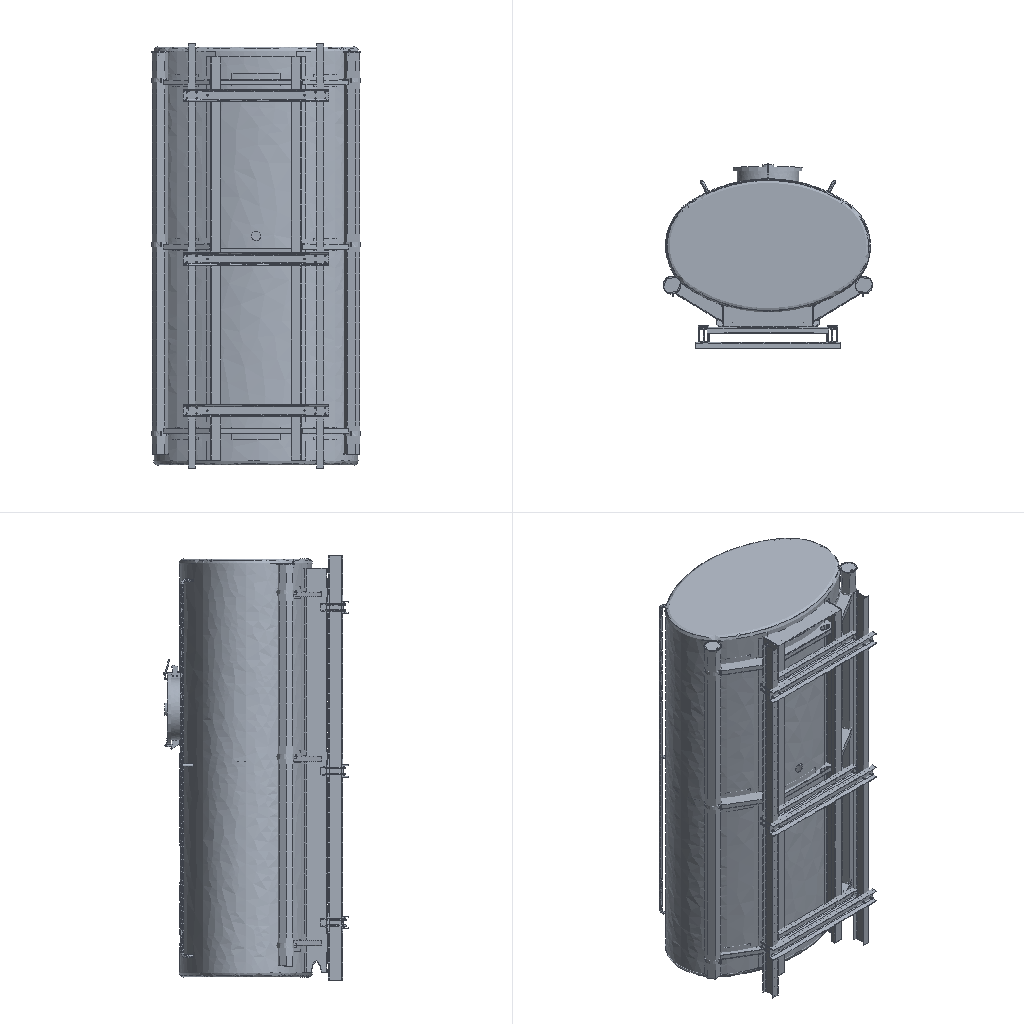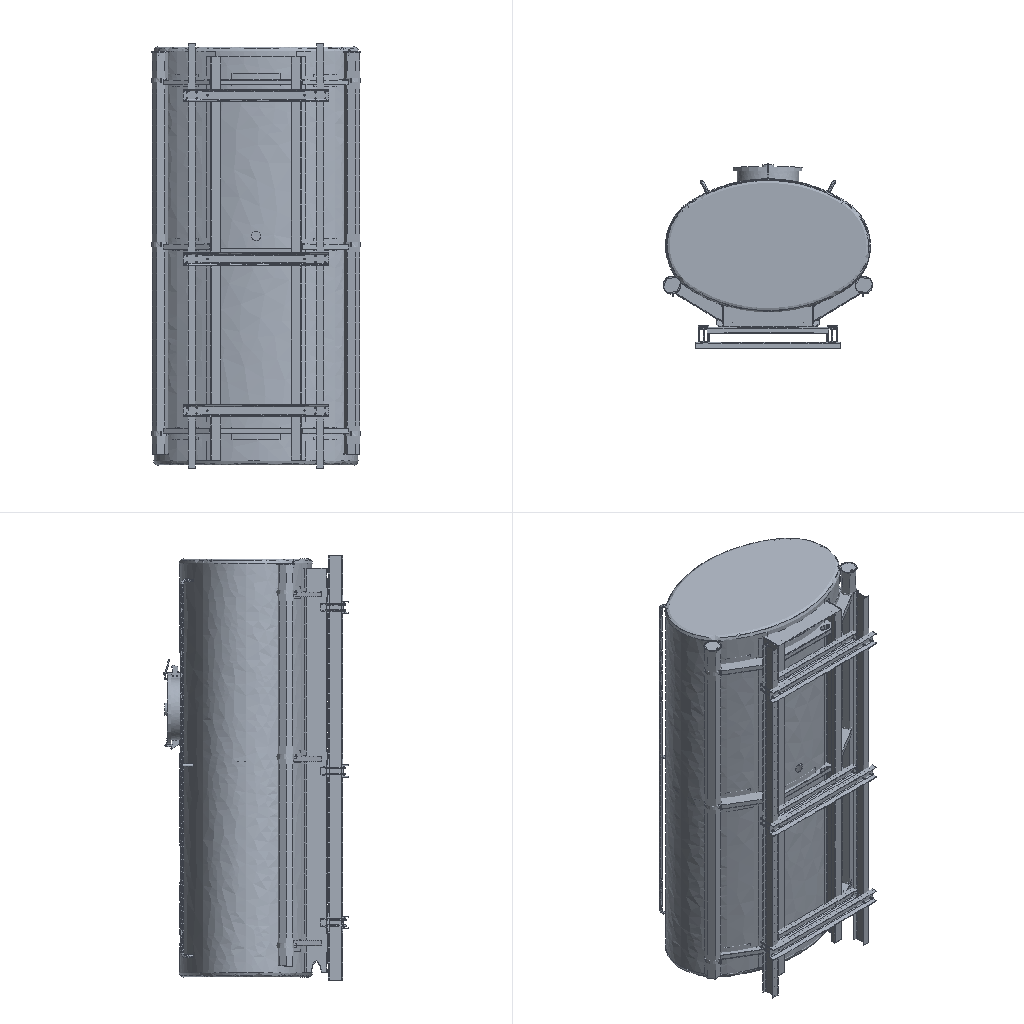Simulation study | ansys workbench
Set-up summary, first 217 of 1807 lines:
category,name,step,type,value,unit,region
solver,ansys_mapdl
solver,version,,,22.1
solver,version,,,22.1
solver,version,,,22.1
units,MPA,,stated
analysis,deck1,,static,static
load_step,requested,,,1
analysis,nlgeom,,,False
mesh,nodes,,,140468
mesh,elements,,,94721
element_type,ANSYS 187 (type 1),,solid,5134
element_type,ANSYS 187 (type 2),,solid,5134
element_type,ANSYS 187 (type 3),,solid,12299
element_type,ANSYS 187 (type 4),,solid,1630
element_type,ANSYS 186 (type 5),,solid,62
element_type,ANSYS 186 (type 6),,solid,48
element_type,ANSYS 187 (type 7),,solid,2207
element_type,ANSYS 187 (type 8),,solid,1194
element_type,ANSYS 186 (type 9),,solid,96
element_type,ANSYS 187 (type 10),,solid,1194
element_type,ANSYS 186 (type 11),,solid,96
element_type,ANSYS 186 (type 12),,solid,252
element_type,ANSYS 187 (type 13),,solid,621
element_type,ANSYS 186 (type 14),,solid,3
element_type,ANSYS 186 (type 15),,solid,21
element_type,ANSYS 186 (type 16),,solid,252
element_type,ANSYS 187 (type 17),,solid,621
element_type,ANSYS 186 (type 18),,solid,3
element_type,ANSYS 186 (type 19),,solid,21
element_type,ANSYS 187 (type 20),,solid,1890
element_type,ANSYS 187 (type 21),,solid,1540
element_type,ANSYS 186 (type 22),,solid,38
element_type,ANSYS 186 (type 23),,solid,68
element_type,ANSYS 186 (type 24),,solid,47
element_type,ANSYS 187 (type 25),,solid,2341
element_type,ANSYS 186 (type 26),,solid,18
element_type,ANSYS 187 (type 27),,solid,2204
element_type,ANSYS 186 (type 28),,solid,18
element_type,ANSYS 186 (type 29),,solid,29
element_type,ANSYS 186 (type 30),,solid,36
element_type,ANSYS 186 (type 31),,solid,36
element_type,ANSYS 187 (type 32),,solid,492
element_type,ANSYS 186 (type 33),,solid,36
element_type,ANSYS 187 (type 34),,solid,492
element_type,ANSYS 187 (type 35),,solid,492
element_type,ANSYS 187 (type 36),,solid,302
element_type,ANSYS 187 (type 37),,solid,297
element_type,ANSYS 187 (type 38),,solid,268
element_type,ANSYS 187 (type 39),,solid,302
element_type,ANSYS 187 (type 40),,solid,302
element_type,ANSYS 187 (type 41),,solid,297
element_type,ANSYS 187 (type 42),,solid,302
element_type,ANSYS 187 (type 43),,solid,268
element_type,ANSYS 187 (type 44),,solid,302
element_type,ANSYS 187 (type 45),,solid,268
element_type,ANSYS 187 (type 46),,solid,302
element_type,ANSYS 187 (type 47),,solid,297
element_type,ANSYS 187 (type 48),,solid,191
element_type,ANSYS 187 (type 49),,solid,191
element_type,ANSYS 187 (type 50),,solid,191
element_type,ANSYS 187 (type 51),,solid,191
element_type,ANSYS 187 (type 52),,solid,191
element_type,ANSYS 187 (type 53),,solid,191
element_type,ANSYS 187 (type 54),,solid,201
element_type,ANSYS 187 (type 55),,solid,201
element_type,ANSYS 187 (type 56),,solid,201
element_type,ANSYS 187 (type 57),,solid,201
element_type,ANSYS 187 (type 58),,solid,201
element_type,ANSYS 187 (type 59),,solid,201
element_type,ANSYS 186 (type 60),,solid,616
element_type,ANSYS 186 (type 61),,solid,616
element_type,ANSYS 187 (type 62),,solid,888
element_type,ANSYS 187 (type 63),,solid,287
element_type,ANSYS 187 (type 64),,solid,287
element_type,ANSYS 187 (type 65),,solid,287
element_type,ANSYS 187 (type 66),,solid,287
element_type,ANSYS 187 (type 67),,solid,1406
element_type,ANSYS 187 (type 68),,solid,888
element_type,ANSYS 187 (type 69),,solid,287
element_type,ANSYS 187 (type 70),,solid,287
element_type,ANSYS 187 (type 71),,solid,287
element_type,ANSYS 187 (type 72),,solid,287
element_type,ANSYS 187 (type 73),,solid,1406
element_type,ANSYS 187 (type 74),,solid,888
element_type,ANSYS 187 (type 75),,solid,287
element_type,ANSYS 187 (type 76),,solid,287
element_type,ANSYS 187 (type 77),,solid,287
element_type,ANSYS 187 (type 78),,solid,287
element_type,ANSYS 187 (type 79),,solid,1406
element_type,ANSYS 174 (type 80),,contact,435
element_type,ANSYS 170 (type 81),,target,435
element_type,ANSYS 174 (type 82),,contact,12
element_type,ANSYS 170 (type 83),,target,12
element_type,ANSYS 174 (type 84),,contact,200
element_type,ANSYS 170 (type 85),,target,200
element_type,ANSYS 174 (type 86),,contact,67
element_type,ANSYS 170 (type 87),,target,67
element_type,ANSYS 174 (type 88),,contact,12
element_type,ANSYS 170 (type 89),,target,12
element_type,ANSYS 174 (type 90),,contact,13
element_type,ANSYS 170 (type 91),,target,13
element_type,ANSYS 174 (type 92),,contact,420
element_type,ANSYS 170 (type 93),,target,420
element_type,ANSYS 174 (type 94),,contact,8
element_type,ANSYS 170 (type 95),,target,8
element_type,ANSYS 174 (type 96),,contact,13
element_type,ANSYS 170 (type 97),,target,13
element_type,ANSYS 174 (type 98),,contact,8
element_type,ANSYS 170 (type 99),,target,8
element_type,ANSYS 174 (type 100),,contact,12
element_type,ANSYS 170 (type 101),,target,12
element_type,ANSYS 174 (type 102),,contact,389
element_type,ANSYS 170 (type 103),,target,389
element_type,ANSYS 174 (type 104),,contact,371
element_type,ANSYS 170 (type 105),,target,371
element_type,ANSYS 174 (type 106),,contact,11
element_type,ANSYS 170 (type 107),,target,11
element_type,ANSYS 174 (type 108),,contact,22
element_type,ANSYS 170 (type 109),,target,22
element_type,ANSYS 174 (type 110),,contact,14
element_type,ANSYS 170 (type 111),,target,14
element_type,ANSYS 174 (type 112),,contact,21
element_type,ANSYS 170 (type 113),,target,21
element_type,ANSYS 174 (type 114),,contact,18
element_type,ANSYS 170 (type 115),,target,18
element_type,ANSYS 174 (type 116),,contact,315
element_type,ANSYS 170 (type 117),,target,315
element_type,ANSYS 174 (type 118),,contact,25
element_type,ANSYS 170 (type 119),,target,25
element_type,ANSYS 174 (type 120),,contact,9
element_type,ANSYS 170 (type 121),,target,9
element_type,ANSYS 174 (type 122),,contact,342
element_type,ANSYS 170 (type 123),,target,342
element_type,ANSYS 174 (type 124),,contact,23
element_type,ANSYS 170 (type 125),,target,23
element_type,ANSYS 174 (type 126),,contact,10
element_type,ANSYS 170 (type 127),,target,10
element_type,ANSYS 174 (type 128),,contact,722
element_type,ANSYS 170 (type 129),,target,722
element_type,ANSYS 174 (type 130),,contact,40
element_type,ANSYS 170 (type 131),,target,40
element_type,ANSYS 174 (type 132),,contact,260
element_type,ANSYS 170 (type 133),,target,260
element_type,ANSYS 174 (type 134),,contact,127
element_type,ANSYS 170 (type 135),,target,127
element_type,ANSYS 174 (type 136),,contact,270
element_type,ANSYS 170 (type 137),,target,270
element_type,ANSYS 174 (type 138),,contact,126
element_type,ANSYS 170 (type 139),,target,126
element_type,ANSYS 174 (type 140),,contact,35
element_type,ANSYS 170 (type 141),,target,35
element_type,ANSYS 174 (type 142),,contact,58
element_type,ANSYS 170 (type 143),,target,58
element_type,ANSYS 174 (type 144),,contact,58
element_type,ANSYS 170 (type 145),,target,58
element_type,ANSYS 174 (type 146),,contact,73
element_type,ANSYS 170 (type 147),,target,73
element_type,ANSYS 174 (type 148),,contact,56
element_type,ANSYS 170 (type 149),,target,56
element_type,ANSYS 174 (type 150),,contact,70
element_type,ANSYS 170 (type 151),,target,70
element_type,ANSYS 174 (type 152),,contact,70
element_type,ANSYS 170 (type 153),,target,70
element_type,ANSYS 174 (type 154),,contact,124
element_type,ANSYS 170 (type 155),,target,124
element_type,ANSYS 174 (type 156),,contact,40
element_type,ANSYS 170 (type 157),,target,40
element_type,ANSYS 174 (type 158),,contact,37
element_type,ANSYS 170 (type 159),,target,37
element_type,ANSYS 174 (type 160),,contact,122
element_type,ANSYS 170 (type 161),,target,122
element_type,ANSYS 174 (type 162),,contact,122
element_type,ANSYS 170 (type 163),,target,122
element_type,ANSYS 174 (type 164),,contact,46
element_type,ANSYS 170 (type 165),,target,46
element_type,ANSYS 174 (type 166),,contact,120
element_type,ANSYS 170 (type 167),,target,120
element_type,ANSYS 174 (type 168),,contact,38
element_type,ANSYS 170 (type 169),,target,38
element_type,ANSYS 174 (type 170),,contact,115
element_type,ANSYS 170 (type 171),,target,115
element_type,ANSYS 174 (type 172),,contact,34
element_type,ANSYS 170 (type 173),,target,34
element_type,ANSYS 174 (type 174),,contact,124
element_type,ANSYS 170 (type 175),,target,124
element_type,ANSYS 174 (type 176),,contact,46
element_type,ANSYS 170 (type 177),,target,46
element_type,ANSYS 174 (type 178),,contact,24
element_type,ANSYS 170 (type 179),,target,24
element_type,ANSYS 174 (type 180),,contact,26
element_type,ANSYS 170 (type 181),,target,26
element_type,ANSYS 174 (type 182),,contact,27
element_type,ANSYS 170 (type 183),,target,27
element_type,ANSYS 174 (type 184),,contact,23
element_type,ANSYS 170 (type 185),,target,23
element_type,ANSYS 174 (type 186),,contact,30
element_type,ANSYS 170 (type 187),,target,30
element_type,ANSYS 174 (type 188),,contact,31
element_type,ANSYS 170 (type 189),,target,31
element_type,ANSYS 174 (type 190),,contact,272
element_type,ANSYS 170 (type 191),,target,272
element_type,ANSYS 174 (type 192),,contact,81
element_type,ANSYS 170 (type 193),,target,81
element_type,ANSYS 174 (type 194),,contact,515
element_type,ANSYS 170 (type 195),,target,515
element_type,ANSYS 174 (type 196),,contact,10
element_type,ANSYS 170 (type 197),,target,10
element_type,ANSYS 174 (type 198),,contact,14
element_type,ANSYS 170 (type 199),,target,14
element_type,ANSYS 174 (type 200),,contact,14
element_type,ANSYS 170 (type 201),,target,14
element_type,ANSYS 174 (type 202),,contact,5
element_type,ANSYS 170 (type 203),,target,5
element_type,ANSYS 174 (type 204),,contact,5
element_type,ANSYS 170 (type 205),,target,5
element_type,ANSYS 174 (type 206),,contact,22
Results summary:
result,analysis,,,static
result,last_loadstep,,,1
result,primary field,,,displacement
result,reaction total,1,FX,714069.728,N
result,reaction total,1,FY,2891340.752,N
result,reaction total,1,FZ,-4.43,N
result,mass,,,1.262,"NMM: mm, ton, N, s, mV, mA, degC"
result,analysis,,,static
result,last_loadstep,,,1
result,primary field,,,displacement
result,reaction total,1,FX,-11.338,N
result,reaction total,1,FY,2503431.821,N
result,reaction total,1,FZ,788430.703,N
result,mass,,,1.262,"NMM: mm, ton, N, s, mV, mA, degC"
result,analysis,,,static
result,last_loadstep,,,1
result,primary field,,,displacement
result,reaction total,1,FX,-0.1212,N
result,reaction total,1,FY,-0.3388,N
result,reaction total,1,FZ,-0.1356,N
result,mass,,,1.262,"NMM: mm, ton, N, s, mV, mA, degC"